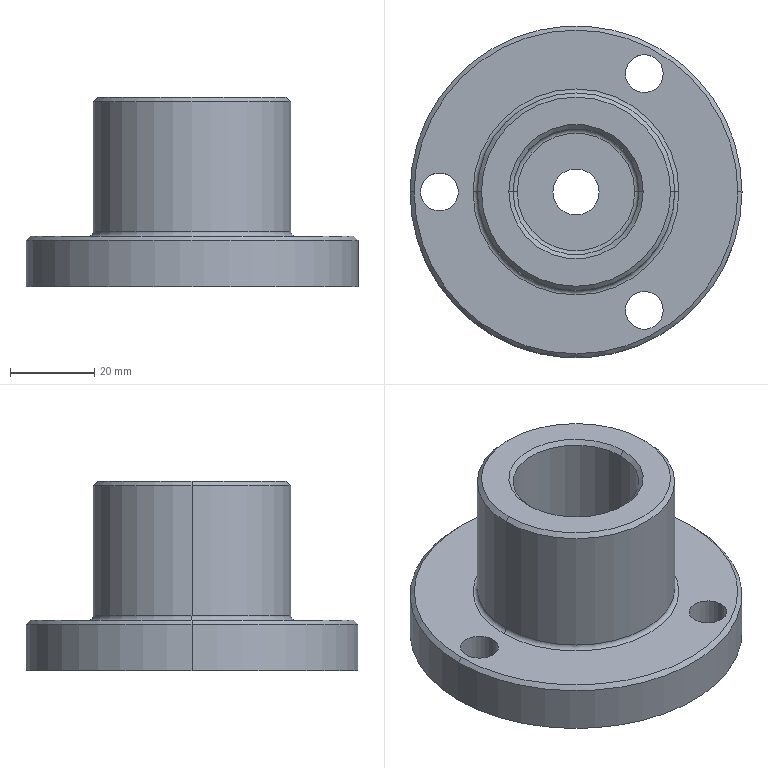Part | SolidWorks | features ICE 5, Chamfer 1, Extrusion 1, Fillet 1 | 1 solid | 30 faces | box 79 x 79 x 45 mm | volume 86695 mm3 | cylinder 14 | cone 8 | torus 4 | plane 4 | commonest cylinder face diameters 9 x6 11 x2 30 x2 47 x2 79 x2
STEP:
#1=CARTESIAN_POINT('',(-23.5,0.,13.));
#2=VERTEX_POINT('',#1);
#3=CARTESIAN_POINT('',(23.5,0.,13.));
#4=VERTEX_POINT('',#3);
#5=CARTESIAN_POINT('',(0.,0.,13.));
#6=DIRECTION('',(0.,0.,1.));
#7=DIRECTION('',(1.,0.,0.));
#8=AXIS2_PLACEMENT_3D('',#5,#6,#7);
#9=CIRCLE('',#8,23.5);
#10=EDGE_CURVE('',#2,#4,#9,.T.);
#11=ORIENTED_EDGE('',*,*,#10,.F.);
#12=CARTESIAN_POINT('',(-24.5,0.,12.));
#13=VERTEX_POINT('',#12);
#14=CARTESIAN_POINT('',(-24.5,0.,13.));
#15=DIRECTION('',(0.,1.,0.));
#16=DIRECTION('',(-1.,0.,0.));
#17=AXIS2_PLACEMENT_3D('',#14,#15,#16);
#18=CIRCLE('',#17,1.);
#19=EDGE_CURVE('',#2,#13,#18,.T.);
#20=ORIENTED_EDGE('',*,*,#19,.T.);
#21=CARTESIAN_POINT('',(24.5,0.,12.));
#22=VERTEX_POINT('',#21);
#23=CARTESIAN_POINT('',(0.,0.,12.));
#24=DIRECTION('',(0.,0.,-1.));
#25=DIRECTION('',(1.,0.,0.));
#26=AXIS2_PLACEMENT_3D('',#23,#24,#25);
#27=CIRCLE('',#26,24.5);
#28=EDGE_CURVE('',#22,#13,#27,.T.);
#29=ORIENTED_EDGE('',*,*,#28,.F.);
#30=CARTESIAN_POINT('',(24.5,0.,13.));
#31=DIRECTION('',(0.,-1.,0.));
#32=DIRECTION('',(0.,0.,-1.));
#33=AXIS2_PLACEMENT_3D('',#30,#31,#32);
#34=CIRCLE('',#33,1.);
#35=EDGE_CURVE('',#4,#22,#34,.T.);
#36=ORIENTED_EDGE('',*,*,#35,.F.);
#37=EDGE_LOOP('',(#11,#20,#29,#36));
#38=FACE_OUTER_BOUND('',#37,.T.);
#39=CARTESIAN_POINT('',(0.,0.,13.));
#40=DIRECTION('',(0.,0.,1.));
#41=DIRECTION('',(1.,0.,0.));
#42=AXIS2_PLACEMENT_3D('',#39,#40,#41);
#43=TOROIDAL_SURFACE('',#42,24.5,1.);
#44=ADVANCED_FACE('',(#38),#43,.F.);
#45=CARTESIAN_POINT('',(-14.,0.,10.));
#46=VERTEX_POINT('',#45);
#47=CARTESIAN_POINT('',(14.,0.,10.));
#48=VERTEX_POINT('',#47);
#49=CARTESIAN_POINT('',(0.,0.,10.));
#50=DIRECTION('',(0.,0.,1.));
#51=DIRECTION('',(1.,0.,0.));
#52=AXIS2_PLACEMENT_3D('',#49,#50,#51);
#53=CIRCLE('',#52,14.);
#54=EDGE_CURVE('',#46,#48,#53,.T.);
#55=ORIENTED_EDGE('',*,*,#54,.F.);
#56=CARTESIAN_POINT('',(-15.,0.,11.));
#57=VERTEX_POINT('',#56);
#58=CARTESIAN_POINT('',(-14.,0.,11.));
#59=DIRECTION('',(0.,1.,0.));
#60=DIRECTION('',(-1.,0.,0.));
#61=AXIS2_PLACEMENT_3D('',#58,#59,#60);
#62=CIRCLE('',#61,1.);
#63=EDGE_CURVE('',#46,#57,#62,.T.);
#64=ORIENTED_EDGE('',*,*,#63,.T.);
#65=CARTESIAN_POINT('',(15.,0.,11.));
#66=VERTEX_POINT('',#65);
#67=CARTESIAN_POINT('',(0.,0.,11.));
#68=DIRECTION('',(0.,0.,-1.));
#69=DIRECTION('',(1.,0.,0.));
#70=AXIS2_PLACEMENT_3D('',#67,#68,#69);
#71=CIRCLE('',#70,15.);
#72=EDGE_CURVE('',#66,#57,#71,.T.);
#73=ORIENTED_EDGE('',*,*,#72,.F.);
#74=CARTESIAN_POINT('',(14.,0.,11.));
#75=DIRECTION('',(0.,-1.,0.));
#76=DIRECTION('',(0.,0.,-1.));
#77=AXIS2_PLACEMENT_3D('',#74,#75,#76);
#78=CIRCLE('',#77,1.);
#79=EDGE_CURVE('',#48,#66,#78,.T.);
#80=ORIENTED_EDGE('',*,*,#79,.F.);
#81=EDGE_LOOP('',(#55,#64,#73,#80));
#82=FACE_OUTER_BOUND('',#81,.T.);
#83=CARTESIAN_POINT('',(0.,0.,11.));
#84=DIRECTION('',(0.,0.,1.));
#85=DIRECTION('',(1.,0.,0.));
#86=AXIS2_PLACEMENT_3D('',#83,#84,#85);
#87=TOROIDAL_SURFACE('',#86,14.,1.);
#88=ADVANCED_FACE('',(#82),#87,.F.);
#89=CARTESIAN_POINT('',(-37.,0.,12.));
#90=VERTEX_POINT('',#89);
#91=CARTESIAN_POINT('',(-28.,0.,12.));
#92=VERTEX_POINT('',#91);
#93=CARTESIAN_POINT('',(-32.5,0.,12.));
#94=DIRECTION('',(0.,0.,1.));
#95=DIRECTION('',(1.,0.,0.));
#96=AXIS2_PLACEMENT_3D('',#93,#94,#95);
#97=CIRCLE('',#96,4.5);
#98=EDGE_CURVE('',#90,#92,#97,.T.);
#99=ORIENTED_EDGE('',*,*,#98,.T.);
#100=CARTESIAN_POINT('',(-28.,0.,0.));
#101=VERTEX_POINT('',#100);
#102=CARTESIAN_POINT('',(-28.,0.,21.));
#103=DIRECTION('',(0.,0.,-1.));
#104=VECTOR('',#103,1000.);
#105=LINE('',#102,#104);
#106=EDGE_CURVE('',#92,#101,#105,.T.);
#107=ORIENTED_EDGE('',*,*,#106,.T.);
#108=CARTESIAN_POINT('',(-37.,0.,0.));
#109=VERTEX_POINT('',#108);
#110=CARTESIAN_POINT('',(-32.5,0.,0.));
#111=DIRECTION('',(0.,0.,-1.));
#112=DIRECTION('',(-1.,0.,0.));
#113=AXIS2_PLACEMENT_3D('',#110,#111,#112);
#114=CIRCLE('',#113,4.5);
#115=EDGE_CURVE('',#101,#109,#114,.T.);
#116=ORIENTED_EDGE('',*,*,#115,.T.);
#117=CARTESIAN_POINT('',(-37.,0.,21.));
#118=DIRECTION('',(0.,0.,-1.));
#119=VECTOR('',#118,1000.);
#120=LINE('',#117,#119);
#121=EDGE_CURVE('',#90,#109,#120,.T.);
#122=ORIENTED_EDGE('',*,*,#121,.F.);
#123=EDGE_LOOP('',(#99,#107,#116,#122));
#124=FACE_OUTER_BOUND('',#123,.T.);
#125=CARTESIAN_POINT('',(-32.5,0.,21.));
#126=DIRECTION('',(0.,0.,-1.));
#127=DIRECTION('',(-1.,0.,0.));
#128=AXIS2_PLACEMENT_3D('',#125,#126,#127);
#129=CYLINDRICAL_SURFACE('',#128,4.5);
#130=ADVANCED_FACE('',(#124),#129,.F.);
#131=CARTESIAN_POINT('',(11.75,-28.146,12.));
#132=VERTEX_POINT('',#131);
#133=CARTESIAN_POINT('',(20.75,-28.146,12.));
#134=VERTEX_POINT('',#133);
#135=CARTESIAN_POINT('',(16.25,-28.146,12.));
#136=DIRECTION('',(0.,0.,1.));
#137=DIRECTION('',(1.,0.,0.));
#138=AXIS2_PLACEMENT_3D('',#135,#136,#137);
#139=CIRCLE('',#138,4.5);
#140=EDGE_CURVE('',#132,#134,#139,.T.);
#141=ORIENTED_EDGE('',*,*,#140,.T.);
#142=CARTESIAN_POINT('',(20.75,-28.146,0.));
#143=VERTEX_POINT('',#142);
#144=CARTESIAN_POINT('',(20.75,-28.146,21.));
#145=DIRECTION('',(0.,0.,-1.));
#146=VECTOR('',#145,1000.);
#147=LINE('',#144,#146);
#148=EDGE_CURVE('',#134,#143,#147,.T.);
#149=ORIENTED_EDGE('',*,*,#148,.T.);
#150=CARTESIAN_POINT('',(11.75,-28.146,0.));
#151=VERTEX_POINT('',#150);
#152=CARTESIAN_POINT('',(16.25,-28.146,0.));
#153=DIRECTION('',(0.,0.,-1.));
#154=DIRECTION('',(-1.,0.,0.));
#155=AXIS2_PLACEMENT_3D('',#152,#153,#154);
#156=CIRCLE('',#155,4.5);
#157=EDGE_CURVE('',#143,#151,#156,.T.);
#158=ORIENTED_EDGE('',*,*,#157,.T.);
#159=CARTESIAN_POINT('',(11.75,-28.146,21.));
#160=DIRECTION('',(0.,0.,-1.));
#161=VECTOR('',#160,1000.);
#162=LINE('',#159,#161);
#163=EDGE_CURVE('',#132,#151,#162,.T.);
#164=ORIENTED_EDGE('',*,*,#163,.F.);
#165=EDGE_LOOP('',(#141,#149,#158,#164));
#166=FACE_OUTER_BOUND('',#165,.T.);
#167=CARTESIAN_POINT('',(16.25,-28.146,21.));
#168=DIRECTION('',(0.,0.,-1.));
#169=DIRECTION('',(-1.,0.,0.));
#170=AXIS2_PLACEMENT_3D('',#167,#168,#169);
#171=CYLINDRICAL_SURFACE('',#170,4.5);
#172=ADVANCED_FACE('',(#166),#171,.F.);
#173=CARTESIAN_POINT('',(11.75,28.146,12.));
#174=VERTEX_POINT('',#173);
#175=CARTESIAN_POINT('',(20.75,28.146,12.));
#176=VERTEX_POINT('',#175);
#177=CARTESIAN_POINT('',(16.25,28.146,12.));
#178=DIRECTION('',(0.,0.,1.));
#179=DIRECTION('',(1.,0.,0.));
#180=AXIS2_PLACEMENT_3D('',#177,#178,#179);
#181=CIRCLE('',#180,4.5);
#182=EDGE_CURVE('',#174,#176,#181,.T.);
#183=ORIENTED_EDGE('',*,*,#182,.T.);
#184=CARTESIAN_POINT('',(20.75,28.146,0.));
#185=VERTEX_POINT('',#184);
#186=CARTESIAN_POINT('',(20.75,28.146,21.));
#187=DIRECTION('',(0.,0.,-1.));
#188=VECTOR('',#187,1000.);
#189=LINE('',#186,#188);
#190=EDGE_CURVE('',#176,#185,#189,.T.);
#191=ORIENTED_EDGE('',*,*,#190,.T.);
#192=CARTESIAN_POINT('',(11.75,28.146,0.));
#193=VERTEX_POINT('',#192);
#194=CARTESIAN_POINT('',(16.25,28.146,0.));
#195=DIRECTION('',(0.,0.,-1.));
#196=DIRECTION('',(-1.,0.,0.));
#197=AXIS2_PLACEMENT_3D('',#194,#195,#196);
#198=CIRCLE('',#197,4.5);
#199=EDGE_CURVE('',#185,#193,#198,.T.);
#200=ORIENTED_EDGE('',*,*,#199,.T.);
#201=CARTESIAN_POINT('',(11.75,28.146,21.));
#202=DIRECTION('',(0.,0.,-1.));
#203=VECTOR('',#202,1000.);
#204=LINE('',#201,#203);
#205=EDGE_CURVE('',#174,#193,#204,.T.);
#206=ORIENTED_EDGE('',*,*,#205,.F.);
#207=EDGE_LOOP('',(#183,#191,#200,#206));
#208=FACE_OUTER_BOUND('',#207,.T.);
#209=CARTESIAN_POINT('',(16.25,28.146,21.));
#210=DIRECTION('',(0.,0.,-1.));
#211=DIRECTION('',(-1.,0.,0.));
#212=AXIS2_PLACEMENT_3D('',#209,#210,#211);
#213=CYLINDRICAL_SURFACE('',#212,4.5);
#214=ADVANCED_FACE('',(#208),#213,.F.);
#215=CARTESIAN_POINT('',(-15.,0.,44.));
#216=VERTEX_POINT('',#215);
#217=CARTESIAN_POINT('',(15.,0.,44.));
#218=VERTEX_POINT('',#217);
#219=CARTESIAN_POINT('',(0.,0.,44.));
#220=DIRECTION('',(0.,0.,1.));
#221=DIRECTION('',(1.,0.,0.));
#222=AXIS2_PLACEMENT_3D('',#219,#220,#221);
#223=CIRCLE('',#222,15.);
#224=EDGE_CURVE('',#216,#218,#223,.T.);
#225=ORIENTED_EDGE('',*,*,#224,.F.);
#226=CARTESIAN_POINT('',(-16.,0.,45.));
#227=VERTEX_POINT('',#226);
#228=CARTESIAN_POINT('',(-15.,0.,44.));
#229=DIRECTION('',(-0.7071,0.,0.7071));
#230=VECTOR('',#229,1000.);
#231=LINE('',#228,#230);
#232=EDGE_CURVE('',#216,#227,#231,.T.);
#233=ORIENTED_EDGE('',*,*,#232,.T.);
#234=CARTESIAN_POINT('',(16.,0.,45.));
#235=VERTEX_POINT('',#234);
#236=CARTESIAN_POINT('',(0.,0.,45.));
#237=DIRECTION('',(0.,0.,-1.));
#238=DIRECTION('',(1.,0.,0.));
#239=AXIS2_PLACEMENT_3D('',#236,#237,#238);
#240=CIRCLE('',#239,16.);
#241=EDGE_CURVE('',#235,#227,#240,.T.);
#242=ORIENTED_EDGE('',*,*,#241,.F.);
#243=CARTESIAN_POINT('',(15.,0.,44.));
#244=DIRECTION('',(0.7071,0.,0.7071));
#245=VECTOR('',#244,1000.);
#246=LINE('',#243,#245);
#247=EDGE_CURVE('',#218,#235,#246,.T.);
#248=ORIENTED_EDGE('',*,*,#247,.F.);
#249=EDGE_LOOP('',(#225,#233,#242,#248));
#250=FACE_OUTER_BOUND('',#249,.T.);
#251=CARTESIAN_POINT('',(0.,0.,44.));
#252=DIRECTION('',(0.,0.,1.));
#253=DIRECTION('',(1.,0.,0.));
#254=AXIS2_PLACEMENT_3D('',#251,#252,#253);
#255=CONICAL_SURFACE('',#254,15.,0.7854);
#256=ADVANCED_FACE('',(#250),#255,.F.);
#257=CARTESIAN_POINT('',(22.5,0.,45.));
#258=VERTEX_POINT('',#257);
#259=CARTESIAN_POINT('',(-22.5,0.,45.));
#260=VERTEX_POINT('',#259);
#261=CARTESIAN_POINT('',(0.,0.,45.));
#262=DIRECTION('',(0.,0.,1.));
#263=DIRECTION('',(1.,0.,0.));
#264=AXIS2_PLACEMENT_3D('',#261,#262,#263);
#265=CIRCLE('',#264,22.5);
#266=EDGE_CURVE('',#258,#260,#265,.T.);
#267=ORIENTED_EDGE('',*,*,#266,.F.);
#268=CARTESIAN_POINT('',(23.5,0.,44.));
#269=VERTEX_POINT('',#268);
#270=CARTESIAN_POINT('',(22.5,0.,45.));
#271=DIRECTION('',(0.7071,0.,-0.7071));
#272=VECTOR('',#271,1000.);
#273=LINE('',#270,#272);
#274=EDGE_CURVE('',#258,#269,#273,.T.);
#275=ORIENTED_EDGE('',*,*,#274,.T.);
#276=CARTESIAN_POINT('',(-23.5,0.,44.));
#277=VERTEX_POINT('',#276);
#278=CARTESIAN_POINT('',(0.,0.,44.));
#279=DIRECTION('',(0.,0.,-1.));
#280=DIRECTION('',(1.,0.,0.));
#281=AXIS2_PLACEMENT_3D('',#278,#279,#280);
#282=CIRCLE('',#281,23.5);
#283=EDGE_CURVE('',#277,#269,#282,.T.);
#284=ORIENTED_EDGE('',*,*,#283,.F.);
#285=CARTESIAN_POINT('',(-22.5,0.,45.));
#286=DIRECTION('',(-0.7071,0.,-0.7071));
#287=VECTOR('',#286,1000.);
#288=LINE('',#285,#287);
#289=EDGE_CURVE('',#260,#277,#288,.T.);
#290=ORIENTED_EDGE('',*,*,#289,.F.);
#291=EDGE_LOOP('',(#267,#275,#284,#290));
#292=FACE_OUTER_BOUND('',#291,.T.);
#293=CARTESIAN_POINT('',(0.,0.,45.));
#294=DIRECTION('',(0.,0.,-1.));
#295=DIRECTION('',(-1.,0.,0.));
#296=AXIS2_PLACEMENT_3D('',#293,#294,#295);
#297=CONICAL_SURFACE('',#296,22.5,0.7854);
#298=ADVANCED_FACE('',(#292),#297,.T.);
#299=CARTESIAN_POINT('',(38.5,0.,12.));
#300=VERTEX_POINT('',#299);
#301=CARTESIAN_POINT('',(-38.5,0.,12.));
#302=VERTEX_POINT('',#301);
#303=CARTESIAN_POINT('',(0.,0.,12.));
#304=DIRECTION('',(0.,0.,1.));
#305=DIRECTION('',(1.,0.,0.));
#306=AXIS2_PLACEMENT_3D('',#303,#304,#305);
#307=CIRCLE('',#306,38.5);
#308=EDGE_CURVE('',#300,#302,#307,.T.);
#309=ORIENTED_EDGE('',*,*,#308,.F.);
#310=CARTESIAN_POINT('',(39.5,0.,11.));
#311=VERTEX_POINT('',#310);
#312=CARTESIAN_POINT('',(38.5,0.,12.));
#313=DIRECTION('',(0.7071,0.,-0.7071));
#314=VECTOR('',#313,1000.);
#315=LINE('',#312,#314);
#316=EDGE_CURVE('',#300,#311,#315,.T.);
#317=ORIENTED_EDGE('',*,*,#316,.T.);
#318=CARTESIAN_POINT('',(-39.5,0.,11.));
#319=VERTEX_POINT('',#318);
#320=CARTESIAN_POINT('',(0.,0.,11.));
#321=DIRECTION('',(0.,0.,-1.));
#322=DIRECTION('',(1.,0.,0.));
#323=AXIS2_PLACEMENT_3D('',#320,#321,#322);
#324=CIRCLE('',#323,39.5);
#325=EDGE_CURVE('',#319,#311,#324,.T.);
#326=ORIENTED_EDGE('',*,*,#325,.F.);
#327=CARTESIAN_POINT('',(-38.5,0.,12.));
#328=DIRECTION('',(-0.7071,0.,-0.7071));
#329=VECTOR('',#328,1000.);
#330=LINE('',#327,#329);
#331=EDGE_CURVE('',#302,#319,#330,.T.);
#332=ORIENTED_EDGE('',*,*,#331,.F.);
#333=EDGE_LOOP('',(#309,#317,#326,#332));
#334=FACE_OUTER_BOUND('',#333,.T.);
#335=CARTESIAN_POINT('',(0.,0.,12.));
#336=DIRECTION('',(0.,0.,-1.));
#337=DIRECTION('',(-1.,0.,0.));
#338=AXIS2_PLACEMENT_3D('',#335,#336,#337);
#339=CONICAL_SURFACE('',#338,38.5,0.7854);
#340=ADVANCED_FACE('',(#334),#339,.T.);
#341=CARTESIAN_POINT('',(5.5,0.,7.));
#342=VERTEX_POINT('',#341);
#343=CARTESIAN_POINT('',(-5.5,0.,7.));
#344=VERTEX_POINT('',#343);
#345=CARTESIAN_POINT('',(0.,0.,7.));
#346=DIRECTION('',(0.,0.,1.));
#347=DIRECTION('',(1.,0.,0.));
#348=AXIS2_PLACEMENT_3D('',#345,#346,#347);
#349=CIRCLE('',#348,5.5);
#350=EDGE_CURVE('',#342,#344,#349,.T.);
#351=ORIENTED_EDGE('',*,*,#350,.T.);
#352=CARTESIAN_POINT('',(-12.5,0.,0.));
#353=VERTEX_POINT('',#352);
#354=CARTESIAN_POINT('',(-5.5,0.,7.));
#355=DIRECTION('',(-0.7071,0.,-0.7071));
#356=VECTOR('',#355,1000.);
#357=LINE('',#354,#356);
#358=EDGE_CURVE('',#344,#353,#357,.T.);
#359=ORIENTED_EDGE('',*,*,#358,.T.);
#360=CARTESIAN_POINT('',(12.5,0.,0.));
#361=VERTEX_POINT('',#360);
#362=CARTESIAN_POINT('',(0.,0.,0.));
#363=DIRECTION('',(0.,0.,1.));
#364=DIRECTION('',(1.,0.,0.));
#365=AXIS2_PLACEMENT_3D('',#362,#363,#364);
#366=CIRCLE('',#365,12.5);
#367=EDGE_CURVE('',#361,#353,#366,.T.);
#368=ORIENTED_EDGE('',*,*,#367,.F.);
#369=CARTESIAN_POINT('',(5.5,0.,7.));
#370=DIRECTION('',(0.7071,0.,-0.7071));
#371=VECTOR('',#370,1000.);
#372=LINE('',#369,#371);
#373=EDGE_CURVE('',#342,#361,#372,.T.);
#374=ORIENTED_EDGE('',*,*,#373,.F.);
#375=EDGE_LOOP('',(#351,#359,#368,#374));
#376=FACE_OUTER_BOUND('',#375,.T.);
#377=CARTESIAN_POINT('',(0.,0.,7.));
#378=DIRECTION('',(0.,0.,-1.));
#379=DIRECTION('',(1.,0.,0.));
#380=AXIS2_PLACEMENT_3D('',#377,#378,#379);
#381=CONICAL_SURFACE('',#380,5.5,0.7854);
#382=ADVANCED_FACE('',(#376),#381,.F.);
#383=CARTESIAN_POINT('',(0.,0.,7.));
#384=DIRECTION('',(0.,0.,1.));
#385=DIRECTION('',(1.,0.,0.));
#386=AXIS2_PLACEMENT_3D('',#383,#384,#385);
#387=CIRCLE('',#386,5.5);
#388=EDGE_CURVE('',#344,#342,#387,.T.);
#389=ORIENTED_EDGE('',*,*,#388,.F.);
#390=CARTESIAN_POINT('',(-5.5,0.,10.));
#391=VERTEX_POINT('',#390);
#392=CARTESIAN_POINT('',(-5.5,0.,7.));
#393=DIRECTION('',(0.,0.,1.));
#394=VECTOR('',#393,1000.);
#395=LINE('',#392,#394);
#396=EDGE_CURVE('',#344,#391,#395,.T.);
#397=ORIENTED_EDGE('',*,*,#396,.T.);
#398=CARTESIAN_POINT('',(5.5,0.,10.));
#399=VERTEX_POINT('',#398);
#400=CARTESIAN_POINT('',(0.,0.,10.));
#401=DIRECTION('',(0.,0.,1.));
#402=DIRECTION('',(1.,0.,0.));
#403=AXIS2_PLACEMENT_3D('',#400,#401,#402);
#404=CIRCLE('',#403,5.5);
#405=EDGE_CURVE('',#391,#399,#404,.T.);
#406=ORIENTED_EDGE('',*,*,#405,.T.);
#407=CARTESIAN_POINT('',(5.5,0.,7.));
#408=DIRECTION('',(0.,0.,1.));
#409=VECTOR('',#408,1000.);
#410=LINE('',#407,#409);
#411=EDGE_CURVE('',#342,#399,#410,.T.);
#412=ORIENTED_EDGE('',*,*,#411,.F.);
#413=EDGE_LOOP('',(#389,#397,#406,#412));
#414=FACE_OUTER_BOUND('',#413,.T.);
#415=CARTESIAN_POINT('',(0.,0.,7.));
#416=DIRECTION('',(0.,0.,1.));
#417=DIRECTION('',(1.,0.,0.));
#418=AXIS2_PLACEMENT_3D('',#415,#416,#417);
#419=CYLINDRICAL_SURFACE('',#418,5.5);
#420=ADVANCED_FACE('',(#414),#419,.F.);
#421=ORIENTED_EDGE('',*,*,#72,.T.);
#422=CARTESIAN_POINT('',(-15.,0.,10.));
#423=DIRECTION('',(0.,0.,1.));
#424=VECTOR('',#423,1000.);
#425=LINE('',#422,#424);
#426=EDGE_CURVE('',#57,#216,#425,.T.);
#427=ORIENTED_EDGE('',*,*,#426,.T.);
#428=ORIENTED_EDGE('',*,*,#224,.T.);
#429=CARTESIAN_POINT('',(15.,0.,10.));
#430=DIRECTION('',(0.,0.,1.));
#431=VECTOR('',#430,1000.);
#432=LINE('',#429,#431);
#433=EDGE_CURVE('',#66,#218,#432,.T.);
#434=ORIENTED_EDGE('',*,*,#433,.F.);
#435=EDGE_LOOP('',(#421,#427,#428,#434));
#436=FACE_OUTER_BOUND('',#435,.T.);
#437=CARTESIAN_POINT('',(0.,0.,10.));
#438=DIRECTION('',(0.,0.,1.));
#439=DIRECTION('',(1.,0.,0.));
#440=AXIS2_PLACEMENT_3D('',#437,#438,#439);
#441=CYLINDRICAL_SURFACE('',#440,15.);
#442=ADVANCED_FACE('',(#436),#441,.F.);
#443=ORIENTED_EDGE('',*,*,#283,.T.);
#444=CARTESIAN_POINT('',(23.5,0.,45.));
#445=DIRECTION('',(0.,0.,-1.));
#446=VECTOR('',#445,1000.);
#447=LINE('',#444,#446);
#448=EDGE_CURVE('',#269,#4,#447,.T.);
#449=ORIENTED_EDGE('',*,*,#448,.T.);
#450=CARTESIAN_POINT('',(0.,0.,13.));
#451=DIRECTION('',(0.,0.,1.));
#452=DIRECTION('',(1.,0.,0.));
#453=AXIS2_PLACEMENT_3D('',#450,#451,#452);
#454=CIRCLE('',#453,23.5);
#455=EDGE_CURVE('',#4,#2,#454,.T.);
#456=ORIENTED_EDGE('',*,*,#455,.T.);
#457=CARTESIAN_POINT('',(-23.5,0.,45.));
#458=DIRECTION('',(0.,0.,-1.));
#459=VECTOR('',#458,1000.);
#460=LINE('',#457,#459);
#461=EDGE_CURVE('',#277,#2,#460,.T.);
#462=ORIENTED_EDGE('',*,*,#461,.F.);
#463=EDGE_LOOP('',(#443,#449,#456,#462));
#464=FACE_OUTER_BOUND('',#463,.T.);
#465=CARTESIAN_POINT('',(0.,0.,45.));
#466=DIRECTION('',(0.,0.,-1.));
#467=DIRECTION('',(-1.,0.,0.));
#468=AXIS2_PLACEMENT_3D('',#465,#466,#467);
#469=CYLINDRICAL_SURFACE('',#468,23.5);
#470=ADVANCED_FACE('',(#464),#469,.T.);
#471=ORIENTED_EDGE('',*,*,#325,.T.);
#472=CARTESIAN_POINT('',(39.5,0.,0.));
#473=VERTEX_POINT('',#472);
#474=CARTESIAN_POINT('',(39.5,0.,12.));
#475=DIRECTION('',(0.,0.,-1.));
#476=VECTOR('',#475,1000.);
#477=LINE('',#474,#476);
#478=EDGE_CURVE('',#311,#473,#477,.T.);
#479=ORIENTED_EDGE('',*,*,#478,.T.);
#480=CARTESIAN_POINT('',(-39.5,0.,0.));
#481=VERTEX_POINT('',#480);
#482=CARTESIAN_POINT('',(0.,0.,0.));
#483=DIRECTION('',(0.,0.,1.));
#484=DIRECTION('',(1.,0.,0.));
#485=AXIS2_PLACEMENT_3D('',#482,#483,#484);
#486=CIRCLE('',#485,39.5);
#487=EDGE_CURVE('',#473,#481,#486,.T.);
#488=ORIENTED_EDGE('',*,*,#487,.T.);
#489=CARTESIAN_POINT('',(-39.5,0.,12.));
#490=DIRECTION('',(0.,0.,-1.));
#491=VECTOR('',#490,1000.);
#492=LINE('',#489,#491);
#493=EDGE_CURVE('',#319,#481,#492,.T.);
#494=ORIENTED_EDGE('',*,*,#493,.F.);
#495=EDGE_LOOP('',(#471,#479,#488,#494));
#496=FACE_OUTER_BOUND('',#495,.T.);
#497=CARTESIAN_POINT('',(0.,0.,12.));
#498=DIRECTION('',(0.,0.,-1.));
#499=DIRECTION('',(-1.,0.,0.));
#500=AXIS2_PLACEMENT_3D('',#497,#498,#499);
#501=CYLINDRICAL_SURFACE('',#500,39.5);
#502=ADVANCED_FACE('',(#496),#501,.T.);
#503=ORIENTED_EDGE('',*,*,#478,.F.);
#504=CARTESIAN_POINT('',(0.,0.,11.));
#505=DIRECTION('',(0.,0.,-1.));
#506=DIRECTION('',(1.,0.,0.));
#507=AXIS2_PLACEMENT_3D('',#504,#505,#506);
#508=CIRCLE('',#507,39.5);
#509=EDGE_CURVE('',#311,#319,#508,.T.);
#510=ORIENTED_EDGE('',*,*,#509,.T.);
#511=ORIENTED_EDGE('',*,*,#493,.T.);
#512=CARTESIAN_POINT('',(0.,0.,0.));
#513=DIRECTION('',(0.,0.,1.));
#514=DIRECTION('',(1.,0.,0.));
#515=AXIS2_PLACEMENT_3D('',#512,#513,#514);
#516=CIRCLE('',#515,39.5);
#517=EDGE_CURVE('',#481,#473,#516,.T.);
#518=ORIENTED_EDGE('',*,*,#517,.T.);
#519=EDGE_LOOP('',(#503,#510,#511,#518));
#520=FACE_OUTER_BOUND('',#519,.T.);
#521=CARTESIAN_POINT('',(0.,0.,12.));
#522=DIRECTION('',(0.,0.,-1.));
#523=DIRECTION('',(-1.,0.,0.));
#524=AXIS2_PLACEMENT_3D('',#521,#522,#523);
#525=CYLINDRICAL_SURFACE('',#524,39.5);
#526=ADVANCED_FACE('',(#520),#525,.T.);
#527=ORIENTED_EDGE('',*,*,#28,.T.);
#528=CARTESIAN_POINT('',(0.,0.,12.));
#529=DIRECTION('',(0.,0.,-1.));
#530=DIRECTION('',(1.,0.,0.));
#531=AXIS2_PLACEMENT_3D('',#528,#529,#530);
#532=CIRCLE('',#531,24.5);
#533=EDGE_CURVE('',#13,#22,#532,.T.);
#534=ORIENTED_EDGE('',*,*,#533,.T.);
#535=EDGE_LOOP('',(#527,#534));
#536=FACE_BOUND('',#535,.T.);
#537=ORIENTED_EDGE('',*,*,#98,.F.);
#538=CARTESIAN_POINT('',(-32.5,0.,12.));
#539=DIRECTION('',(0.,0.,1.));
#540=DIRECTION('',(1.,0.,0.));
#541=AXIS2_PLACEMENT_3D('',#538,#539,#540);
#542=CIRCLE('',#541,4.5);
#543=EDGE_CURVE('',#92,#90,#542,.T.);
#544=ORIENTED_EDGE('',*,*,#543,.F.);
#545=EDGE_LOOP('',(#537,#544));
#546=FACE_BOUND('',#545,.T.);
#547=ORIENTED_EDGE('',*,*,#140,.F.);
#548=CARTESIAN_POINT('',(16.25,-28.146,12.));
#549=DIRECTION('',(0.,0.,1.));
#550=DIRECTION('',(1.,0.,0.));
#551=AXIS2_PLACEMENT_3D('',#548,#549,#550);
#552=CIRCLE('',#551,4.5);
#553=EDGE_CURVE('',#134,#132,#552,.T.);
#554=ORIENTED_EDGE('',*,*,#553,.F.);
#555=EDGE_LOOP('',(#547,#554));
#556=FACE_BOUND('',#555,.T.);
#557=ORIENTED_EDGE('',*,*,#182,.F.);
#558=CARTESIAN_POINT('',(16.25,28.146,12.));
#559=DIRECTION('',(0.,0.,1.));
#560=DIRECTION('',(1.,0.,0.));
#561=AXIS2_PLACEMENT_3D('',#558,#559,#560);
#562=CIRCLE('',#561,4.5);
#563=EDGE_CURVE('',#176,#174,#562,.T.);
#564=ORIENTED_EDGE('',*,*,#563,.F.);
#565=EDGE_LOOP('',(#557,#564));
#566=FACE_BOUND('',#565,.T.);
#567=CARTESIAN_POINT('',(0.,0.,12.));
#568=DIRECTION('',(0.,0.,1.));
#569=DIRECTION('',(1.,0.,0.));
#570=AXIS2_PLACEMENT_3D('',#567,#568,#569);
#571=CIRCLE('',#570,38.5);
#572=EDGE_CURVE('',#302,#300,#571,.T.);
#573=ORIENTED_EDGE('',*,*,#572,.T.);
#574=ORIENTED_EDGE('',*,*,#308,.T.);
#575=EDGE_LOOP('',(#573,#574));
#576=FACE_OUTER_BOUND('',#575,.T.);
#577=CARTESIAN_POINT('',(0.,0.,12.));
#578=DIRECTION('',(0.,0.,1.));
#579=DIRECTION('',(1.,0.,0.));
#580=AXIS2_PLACEMENT_3D('',#577,#578,#579);
#581=PLANE('',#580);
#582=ADVANCED_FACE('',(#536,#546,#556,#566,#576),#581,.T.);
#583=CARTESIAN_POINT('',(-32.5,0.,0.));
#584=DIRECTION('',(0.,0.,-1.));
#585=DIRECTION('',(-1.,0.,0.));
#586=AXIS2_PLACEMENT_3D('',#583,#584,#585);
#587=CIRCLE('',#586,4.5);
#588=EDGE_CURVE('',#109,#101,#587,.T.);
#589=ORIENTED_EDGE('',*,*,#588,.F.);
#590=ORIENTED_EDGE('',*,*,#115,.F.);
#591=EDGE_LOOP('',(#589,#590));
#592=FACE_BOUND('',#591,.T.);
#593=CARTESIAN_POINT('',(16.25,-28.146,0.));
#594=DIRECTION('',(0.,0.,-1.));
#595=DIRECTION('',(-1.,0.,0.));
#596=AXIS2_PLACEMENT_3D('',#593,#594,#595);
#597=CIRCLE('',#596,4.5);
#598=EDGE_CURVE('',#151,#143,#597,.T.);
#599=ORIENTED_EDGE('',*,*,#598,.F.);
#600=ORIENTED_EDGE('',*,*,#157,.F.);
#601=EDGE_LOOP('',(#599,#600));
#602=FACE_BOUND('',#601,.T.);
#603=CARTESIAN_POINT('',(16.25,28.146,0.));
#604=DIRECTION('',(0.,0.,-1.));
#605=DIRECTION('',(-1.,0.,0.));
#606=AXIS2_PLACEMENT_3D('',#603,#604,#605);
#607=CIRCLE('',#606,4.5);
#608=EDGE_CURVE('',#193,#185,#607,.T.);
#609=ORIENTED_EDGE('',*,*,#608,.F.);
#610=ORIENTED_EDGE('',*,*,#199,.F.);
#611=EDGE_LOOP('',(#609,#610));
#612=FACE_BOUND('',#611,.T.);
#613=ORIENTED_EDGE('',*,*,#367,.T.);
#614=CARTESIAN_POINT('',(0.,0.,0.));
#615=DIRECTION('',(0.,0.,1.));
#616=DIRECTION('',(1.,0.,0.));
#617=AXIS2_PLACEMENT_3D('',#614,#615,#616);
#618=CIRCLE('',#617,12.5);
#619=EDGE_CURVE('',#353,#361,#618,.T.);
#620=ORIENTED_EDGE('',*,*,#619,.T.);
#621=EDGE_LOOP('',(#613,#620));
#622=FACE_BOUND('',#621,.T.);
#623=ORIENTED_EDGE('',*,*,#517,.F.);
#624=ORIENTED_EDGE('',*,*,#487,.F.);
#625=EDGE_LOOP('',(#623,#624));
#626=FACE_OUTER_BOUND('',#625,.T.);
#627=CARTESIAN_POINT('',(0.,0.,0.));
#628=DIRECTION('',(0.,0.,1.));
#629=DIRECTION('',(1.,0.,0.));
#630=AXIS2_PLACEMENT_3D('',#627,#628,#629);
#631=PLANE('',#630);
#632=ADVANCED_FACE('',(#592,#602,#612,#622,#626),#631,.F.);
#633=ORIENTED_EDGE('',*,*,#448,.F.);
#634=CARTESIAN_POINT('',(0.,0.,44.));
#635=DIRECTION('',(0.,0.,-1.));
#636=DIRECTION('',(1.,0.,0.));
#637=AXIS2_PLACEMENT_3D('',#634,#635,#636);
#638=CIRCLE('',#637,23.5);
#639=EDGE_CURVE('',#269,#277,#638,.T.);
#640=ORIENTED_EDGE('',*,*,#639,.T.);
#641=ORIENTED_EDGE('',*,*,#461,.T.);
#642=ORIENTED_EDGE('',*,*,#10,.T.);
#643=EDGE_LOOP('',(#633,#640,#641,#642));
#644=FACE_OUTER_BOUND('',#643,.T.);
#645=CARTESIAN_POINT('',(0.,0.,45.));
#646=DIRECTION('',(0.,0.,-1.));
#647=DIRECTION('',(-1.,0.,0.));
#648=AXIS2_PLACEMENT_3D('',#645,#646,#647);
#649=CYLINDRICAL_SURFACE('',#648,23.5);
#650=ADVANCED_FACE('',(#644),#649,.T.);
#651=CARTESIAN_POINT('',(0.,0.,45.));
#652=DIRECTION('',(0.,0.,1.));
#653=DIRECTION('',(1.,0.,0.));
#654=AXIS2_PLACEMENT_3D('',#651,#652,#653);
#655=CIRCLE('',#654,22.5);
#656=EDGE_CURVE('',#260,#258,#655,.T.);
#657=ORIENTED_EDGE('',*,*,#656,.T.);
#658=ORIENTED_EDGE('',*,*,#266,.T.);
#659=EDGE_LOOP('',(#657,#658));
#660=FACE_OUTER_BOUND('',#659,.T.);
#661=ORIENTED_EDGE('',*,*,#241,.T.);
#662=CARTESIAN_POINT('',(0.,0.,45.));
#663=DIRECTION('',(0.,0.,-1.));
#664=DIRECTION('',(1.,0.,0.));
#665=AXIS2_PLACEMENT_3D('',#662,#663,#664);
#666=CIRCLE('',#665,16.);
#667=EDGE_CURVE('',#227,#235,#666,.T.);
#668=ORIENTED_EDGE('',*,*,#667,.T.);
#669=EDGE_LOOP('',(#661,#668));
#670=FACE_BOUND('',#669,.T.);
#671=CARTESIAN_POINT('',(0.,0.,45.));
#672=DIRECTION('',(0.,0.,1.));
#673=DIRECTION('',(1.,0.,0.));
#674=AXIS2_PLACEMENT_3D('',#671,#672,#673);
#675=PLANE('',#674);
#676=ADVANCED_FACE('',(#660,#670),#675,.T.);
#677=ORIENTED_EDGE('',*,*,#426,.F.);
#678=CARTESIAN_POINT('',(0.,0.,11.));
#679=DIRECTION('',(0.,0.,-1.));
#680=DIRECTION('',(1.,0.,0.));
#681=AXIS2_PLACEMENT_3D('',#678,#679,#680);
#682=CIRCLE('',#681,15.);
#683=EDGE_CURVE('',#57,#66,#682,.T.);
#684=ORIENTED_EDGE('',*,*,#683,.T.);
#685=ORIENTED_EDGE('',*,*,#433,.T.);
#686=CARTESIAN_POINT('',(0.,0.,44.));
#687=DIRECTION('',(0.,0.,1.));
#688=DIRECTION('',(1.,0.,0.));
#689=AXIS2_PLACEMENT_3D('',#686,#687,#688);
#690=CIRCLE('',#689,15.);
#691=EDGE_CURVE('',#218,#216,#690,.T.);
#692=ORIENTED_EDGE('',*,*,#691,.T.);
#693=EDGE_LOOP('',(#677,#684,#685,#692));
#694=FACE_OUTER_BOUND('',#693,.T.);
#695=CARTESIAN_POINT('',(0.,0.,10.));
#696=DIRECTION('',(0.,0.,1.));
#697=DIRECTION('',(1.,0.,0.));
#698=AXIS2_PLACEMENT_3D('',#695,#696,#697);
#699=CYLINDRICAL_SURFACE('',#698,15.);
#700=ADVANCED_FACE('',(#694),#699,.F.);
#701=CARTESIAN_POINT('',(0.,0.,10.));
#702=DIRECTION('',(0.,0.,1.));
#703=DIRECTION('',(1.,0.,0.));
#704=AXIS2_PLACEMENT_3D('',#701,#702,#703);
#705=CIRCLE('',#704,14.);
#706=EDGE_CURVE('',#48,#46,#705,.T.);
#707=ORIENTED_EDGE('',*,*,#706,.T.);
#708=ORIENTED_EDGE('',*,*,#54,.T.);
#709=EDGE_LOOP('',(#707,#708));
#710=FACE_OUTER_BOUND('',#709,.T.);
#711=CARTESIAN_POINT('',(0.,0.,10.));
#712=DIRECTION('',(0.,0.,1.));
#713=DIRECTION('',(1.,0.,0.));
#714=AXIS2_PLACEMENT_3D('',#711,#712,#713);
#715=CIRCLE('',#714,5.5);
#716=EDGE_CURVE('',#399,#391,#715,.T.);
#717=ORIENTED_EDGE('',*,*,#716,.F.);
#718=ORIENTED_EDGE('',*,*,#405,.F.);
#719=EDGE_LOOP('',(#717,#718));
#720=FACE_BOUND('',#719,.T.);
#721=CARTESIAN_POINT('',(0.,0.,10.));
#722=DIRECTION('',(0.,0.,1.));
#723=DIRECTION('',(1.,0.,0.));
#724=AXIS2_PLACEMENT_3D('',#721,#722,#723);
#725=PLANE('',#724);
#726=ADVANCED_FACE('',(#710,#720),#725,.T.);
#727=ORIENTED_EDGE('',*,*,#396,.F.);
#728=ORIENTED_EDGE('',*,*,#350,.F.);
#729=ORIENTED_EDGE('',*,*,#411,.T.);
#730=ORIENTED_EDGE('',*,*,#716,.T.);
#731=EDGE_LOOP('',(#727,#728,#729,#730));
#732=FACE_OUTER_BOUND('',#731,.T.);
#733=CARTESIAN_POINT('',(0.,0.,7.));
#734=DIRECTION('',(0.,0.,1.));
#735=DIRECTION('',(1.,0.,0.));
#736=AXIS2_PLACEMENT_3D('',#733,#734,#735);
#737=CYLINDRICAL_SURFACE('',#736,5.5);
#738=ADVANCED_FACE('',(#732),#737,.F.);
#739=ORIENTED_EDGE('',*,*,#358,.F.);
#740=ORIENTED_EDGE('',*,*,#388,.T.);
#741=ORIENTED_EDGE('',*,*,#373,.T.);
#742=ORIENTED_EDGE('',*,*,#619,.F.);
#743=EDGE_LOOP('',(#739,#740,#741,#742));
#744=FACE_OUTER_BOUND('',#743,.T.);
#745=CARTESIAN_POINT('',(0.,0.,7.));
#746=DIRECTION('',(0.,0.,-1.));
#747=DIRECTION('',(1.,0.,0.));
#748=AXIS2_PLACEMENT_3D('',#745,#746,#747);
#749=CONICAL_SURFACE('',#748,5.5,0.7854);
#750=ADVANCED_FACE('',(#744),#749,.F.);
#751=ORIENTED_EDGE('',*,*,#316,.F.);
#752=ORIENTED_EDGE('',*,*,#572,.F.);
#753=ORIENTED_EDGE('',*,*,#331,.T.);
#754=ORIENTED_EDGE('',*,*,#509,.F.);
#755=EDGE_LOOP('',(#751,#752,#753,#754));
#756=FACE_OUTER_BOUND('',#755,.T.);
#757=CARTESIAN_POINT('',(0.,0.,12.));
#758=DIRECTION('',(0.,0.,-1.));
#759=DIRECTION('',(-1.,0.,0.));
#760=AXIS2_PLACEMENT_3D('',#757,#758,#759);
#761=CONICAL_SURFACE('',#760,38.5,0.7854);
#762=ADVANCED_FACE('',(#756),#761,.T.);
#763=ORIENTED_EDGE('',*,*,#274,.F.);
#764=ORIENTED_EDGE('',*,*,#656,.F.);
#765=ORIENTED_EDGE('',*,*,#289,.T.);
#766=ORIENTED_EDGE('',*,*,#639,.F.);
#767=EDGE_LOOP('',(#763,#764,#765,#766));
#768=FACE_OUTER_BOUND('',#767,.T.);
#769=CARTESIAN_POINT('',(0.,0.,45.));
#770=DIRECTION('',(0.,0.,-1.));
#771=DIRECTION('',(-1.,0.,0.));
#772=AXIS2_PLACEMENT_3D('',#769,#770,#771);
#773=CONICAL_SURFACE('',#772,22.5,0.7854);
#774=ADVANCED_FACE('',(#768),#773,.T.);
#775=ORIENTED_EDGE('',*,*,#232,.F.);
#776=ORIENTED_EDGE('',*,*,#691,.F.);
#777=ORIENTED_EDGE('',*,*,#247,.T.);
#778=ORIENTED_EDGE('',*,*,#667,.F.);
#779=EDGE_LOOP('',(#775,#776,#777,#778));
#780=FACE_OUTER_BOUND('',#779,.T.);
#781=CARTESIAN_POINT('',(0.,0.,44.));
#782=DIRECTION('',(0.,0.,1.));
#783=DIRECTION('',(1.,0.,0.));
#784=AXIS2_PLACEMENT_3D('',#781,#782,#783);
#785=CONICAL_SURFACE('',#784,15.,0.7854);
#786=ADVANCED_FACE('',(#780),#785,.F.);
#787=ORIENTED_EDGE('',*,*,#190,.F.);
#788=ORIENTED_EDGE('',*,*,#563,.T.);
#789=ORIENTED_EDGE('',*,*,#205,.T.);
#790=ORIENTED_EDGE('',*,*,#608,.T.);
#791=EDGE_LOOP('',(#787,#788,#789,#790));
#792=FACE_OUTER_BOUND('',#791,.T.);
#793=CARTESIAN_POINT('',(16.25,28.146,21.));
#794=DIRECTION('',(0.,0.,-1.));
#795=DIRECTION('',(-1.,0.,0.));
#796=AXIS2_PLACEMENT_3D('',#793,#794,#795);
#797=CYLINDRICAL_SURFACE('',#796,4.5);
#798=ADVANCED_FACE('',(#792),#797,.F.);
#799=ORIENTED_EDGE('',*,*,#148,.F.);
#800=ORIENTED_EDGE('',*,*,#553,.T.);
#801=ORIENTED_EDGE('',*,*,#163,.T.);
#802=ORIENTED_EDGE('',*,*,#598,.T.);
#803=EDGE_LOOP('',(#799,#800,#801,#802));
#804=FACE_OUTER_BOUND('',#803,.T.);
#805=CARTESIAN_POINT('',(16.25,-28.146,21.));
#806=DIRECTION('',(0.,0.,-1.));
#807=DIRECTION('',(-1.,0.,0.));
#808=AXIS2_PLACEMENT_3D('',#805,#806,#807);
#809=CYLINDRICAL_SURFACE('',#808,4.5);
#810=ADVANCED_FACE('',(#804),#809,.F.);
#811=ORIENTED_EDGE('',*,*,#106,.F.);
#812=ORIENTED_EDGE('',*,*,#543,.T.);
#813=ORIENTED_EDGE('',*,*,#121,.T.);
#814=ORIENTED_EDGE('',*,*,#588,.T.);
#815=EDGE_LOOP('',(#811,#812,#813,#814));
#816=FACE_OUTER_BOUND('',#815,.T.);
#817=CARTESIAN_POINT('',(-32.5,0.,21.));
#818=DIRECTION('',(0.,0.,-1.));
#819=DIRECTION('',(-1.,0.,0.));
#820=AXIS2_PLACEMENT_3D('',#817,#818,#819);
#821=CYLINDRICAL_SURFACE('',#820,4.5);
#822=ADVANCED_FACE('',(#816),#821,.F.);
#823=ORIENTED_EDGE('',*,*,#63,.F.);
#824=ORIENTED_EDGE('',*,*,#706,.F.);
#825=ORIENTED_EDGE('',*,*,#79,.T.);
#826=ORIENTED_EDGE('',*,*,#683,.F.);
#827=EDGE_LOOP('',(#823,#824,#825,#826));
#828=FACE_OUTER_BOUND('',#827,.T.);
#829=CARTESIAN_POINT('',(0.,0.,11.));
#830=DIRECTION('',(0.,0.,1.));
#831=DIRECTION('',(1.,0.,0.));
#832=AXIS2_PLACEMENT_3D('',#829,#830,#831);
#833=TOROIDAL_SURFACE('',#832,14.,1.);
#834=ADVANCED_FACE('',(#828),#833,.F.);
#835=ORIENTED_EDGE('',*,*,#19,.F.);
#836=ORIENTED_EDGE('',*,*,#455,.F.);
#837=ORIENTED_EDGE('',*,*,#35,.T.);
#838=ORIENTED_EDGE('',*,*,#533,.F.);
#839=EDGE_LOOP('',(#835,#836,#837,#838));
#840=FACE_OUTER_BOUND('',#839,.T.);
#841=CARTESIAN_POINT('',(0.,0.,13.));
#842=DIRECTION('',(0.,0.,1.));
#843=DIRECTION('',(1.,0.,0.));
#844=AXIS2_PLACEMENT_3D('',#841,#842,#843);
#845=TOROIDAL_SURFACE('',#844,24.5,1.);
#846=ADVANCED_FACE('',(#840),#845,.F.);
#847=CLOSED_SHELL('',(#44,#88,#130,#172,#214,#256,#298,#340,#382,#420,#442,#470,#502,#526,#582,#632,#650,#676,#700,#726,#738,#750,#762,#774,#786,#798,#810,#822,#834,#846));
#848=MANIFOLD_SOLID_BREP('',#847);
#849=CARTESIAN_POINT('',(0.,0.,0.));
#850=DIRECTION('',(0.,0.,1.));
#851=DIRECTION('',(1.,0.,0.));
#852=AXIS2_PLACEMENT_3D('',#849,#850,#851);
#853=(LENGTH_UNIT()NAMED_UNIT(*)SI_UNIT(.MILLI.,.METRE.));
#854=UNCERTAINTY_MEASURE_WITH_UNIT(LENGTH_MEASURE(0.00001),#853,'','');
#855=(NAMED_UNIT(*)PLANE_ANGLE_UNIT()SI_UNIT($,.RADIAN.));
#856=(NAMED_UNIT(*)SI_UNIT($,.STERADIAN.)SOLID_ANGLE_UNIT());
#857=(GEOMETRIC_REPRESENTATION_CONTEXT(3)GLOBAL_UNCERTAINTY_ASSIGNED_CONTEXT((#854))GLOBAL_UNIT_ASSIGNED_CONTEXT((#853,#855,#856))REPRESENTATION_CONTEXT('',''));
#858=ADVANCED_BREP_SHAPE_REPRESENTATION('',(#848,#852),#857);